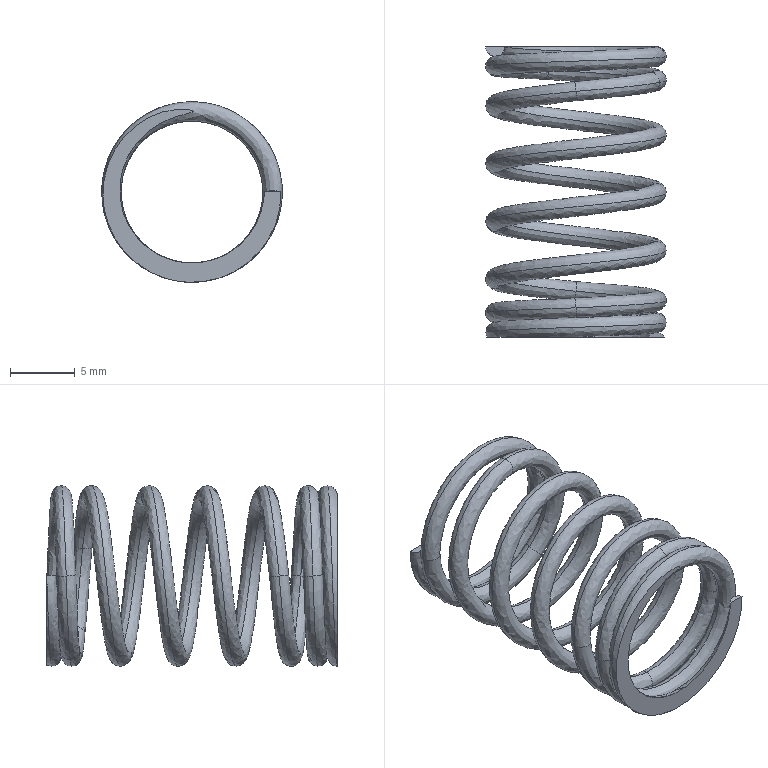Part | STEP file | Compress Spring1_2 | 1 solid | 26 faces | volume 492.963 mm3 | spline 22 | plane 4